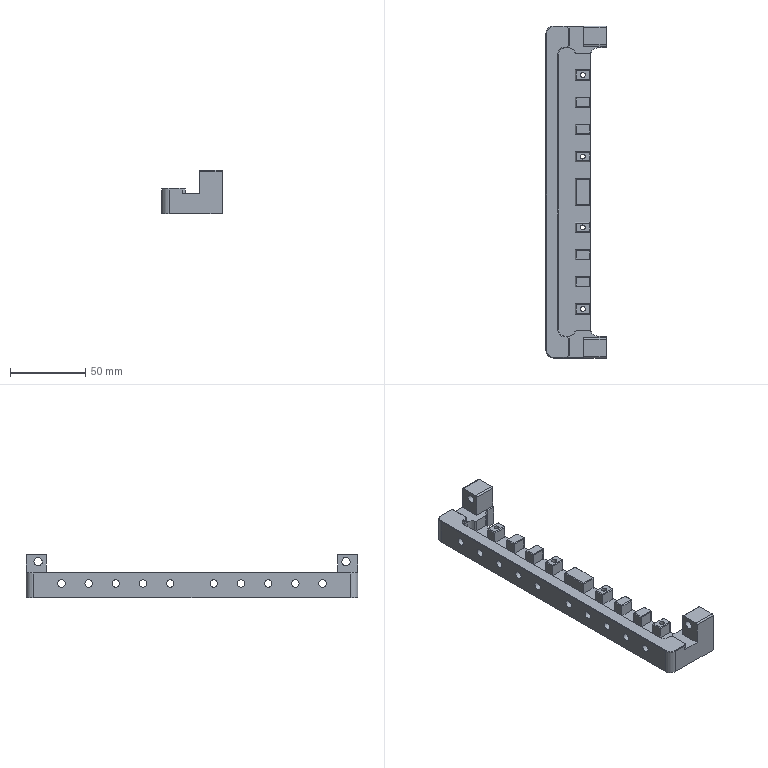CAM job | NX | 3-axis milling, drilling | part box 40 x 220 x 29 mm | stock box 45 x 225 x 35 mm
Tools:
number,name,description,diameter,corner_radius,flute_length,length,flutes
6,D6,平底铣刀-粗,6.0,0.0,25.0,75.0,2
9,D10,平底铣刀-粗,10.0,0.0,35.0,75.0,2
7,D6-J,平底铣刀-精,6.0,0.0,25.0,75.0,2
10,D10-J,平底铣刀-精,10.0,0.0,35.0,75.0,2
17,D6R0.5,圆鼻刀-粗,6.0,0.5,50.0,75.0,2
1,D80R0.8飞刀,圆鼻刀-粗,80.0,0.8,50.0,75.0,2
1,D80R0.8飞刀-J,圆鼻刀-精,80.0,0.8,50.0,75.0,2
2,D6倒角刀,倒角刀,6.0,0.0,3.0,25.0,2
21,M4X0.7,丝锥,3.3,0.0,35.0,50.0,2
13,钻头3.3,Twist Drill 3.3 mm,3.3,0.0,35.0,35.008,2
Operations:
program,operation,operation_type,tool,method,geometry_group,spindle_rpm,surface_speed,feed_per_tooth,feed_cut,feed_plunge,cut_length_mm,path_length_mm,cut_time_min,machine_time_min
B,底壁铣飞面一刀开粗_COPY,VolumeBased25DMillingOperation,D80R0.8飞刀,分层开粗-切深K-步距G,W-B,2800.0,703.696,0.5357,3000.0,100.0,3938.598,7791.555,1.313,1.698
B,底壁铣飞面一刀精光_COPY,VolumeBased25DMillingOperation,D80R0.8飞刀-J,侧刃精光-切深K-步距G,W-B,4000.0,1005.28,0.125,1000.0,100.0,328.021,364.021,0.328,0.3316
B,底壁铣分层开粗-中_COPY,VolumeBased25DMillingOperation,D10,分层开粗-切深K-步距G,W-B,8000.0,251.32,0.25,4000.0,100.0,35394.52,36209.865,8.849,8.93
B,底壁铣分层开粗-中_COPY_1,VolumeBased25DMillingOperation,D10,分层开粗-切深K-步距G,W-B,8000.0,251.32,0.25,4000.0,100.0,17945.335,18024.488,4.486,4.494
B,底壁铣分层开粗-中_COPY_2,VolumeBased25DMillingOperation,D6,分层开粗-切深K-步距G,W-B,8000.0,150.792,0.1875,3000.0,100.0,1582.336,1826.173,0.5274,0.5518
B,等高光顺清角D6参考12_COPY,ZLevelMilling,D6-J,分层精光-切深K-步距G,W-B,8000.0,150.792,0.075,1200.0,100.0,1057.613,1361.457,0.8813,0.9117
B,等高精光往复爬面_COPY,ZLevelMilling,D6R0.5,等高爬面-切深K-步距G,W-B,7000.0,131.947,0.3214,4500.0,100.0,1750.97,2143.172,0.3891,0.4283
B,钻倒角_2,Operation,D6倒角刀,METHOD,W-B,8000.0,150.796,0.0625,1000.0,0.0,20.8,276.862,0.0208,0.0464
B,平面去毛刺6X45L_COPY,SurfaceContour,D6倒角刀,爬面_倒角-切深0-步距G,W-B,6500.0,122.519,0.1154,1500.0,100.0,406.96,2498.027,0.2713,0.4804
B,平面去毛刺6X45L_COPY_1,SurfaceContour,D6倒角刀,爬面_倒角-切深0-步距G,W-B,6500.0,122.519,0.1154,1500.0,100.0,971.496,1644.992,0.6477,0.715
B,底壁铣精光底面-中_COPY,VolumeBased25DMillingOperation,D6-J,精光步距切深关,W-B,8000.0,150.792,0.0625,1000.0,100.0,74.03,133.63,0.074,0.08
B,底壁铣精光底面-中_COPY_4,VolumeBased25DMillingOperation,D6-J,精光步距切深关,W-B,7000.0,175.0,0.0536,1500.0,100.0,975.502,1028.102,0.6503,0.6556
B,底壁铣精光底面-中_COPY_3,VolumeBased25DMillingOperation,D6-J,精光步距切深关,W-B,7000.0,175.0,0.0536,1500.0,100.0,625.075,799.403,0.4167,0.4341
B,底壁铣精光底面-中_COPY_1,VolumeBased25DMillingOperation,D6-J,精光步距切深关,W-B,7000.0,175.0,0.0536,1500.0,100.0,74.03,133.63,0.0494,0.0553
B,底壁铣精光底面-中_COPY_2,VolumeBased25DMillingOperation,D6-J,精光步距切深关,W-B,8000.0,150.792,0.0625,1000.0,100.0,681.584,757.384,0.6816,0.6892
B,底壁铣精光侧面-中_COPY,VolumeBased25DMillingOperation,D6-J,侧刃精光-切深K-步距G,W-B,8000.0,150.792,0.0625,1000.0,100.0,74.707,481.632,0.0747,0.1154
B,底壁铣精光侧面-中_COPY_1,VolumeBased25DMillingOperation,D6-J,侧刃精光-切深K-步距G,W-B,8000.0,150.792,0.0625,1000.0,100.0,280.153,860.83,0.2802,0.3382
B,底壁铣精光侧面-中-选底面_COPY,VolumeBased25DMillingOperation,D6-J,侧刃精光-切深K-步距G,W-B,8000.0,150.792,0.0625,1000.0,100.0,747.836,955.024,0.7478,0.7686
A,顶面,FaceMilling,D80R0.8飞刀,侧刃精光-切深K-步距G,W-A,5000.0,1256.637,0.1,1000.0,100.0,314.0,350.0,0.314,0.3176
A,动态开粗D10_COPY,CavityMilling,D10,动态开粗-切深K-步距K,W-A,8000.0,251.32,0.25,4000.0,100.0,11970.014,12931.832,2.993,3.089
A,打点-深0.8,Operation,D6倒角刀,NONE,W-A,8000.0,150.796,0.0312,500.0,90.0,7.2,212.429,0.0144,0.0349
A,通孔-M4螺纹底孔,Operation,钻头3.3,NONE,W-A,3000.0,31.102,0.05,300.0,90.0,92.0,382.029,0.3067,0.3357
A,仅选体,SurfaceContour,D6倒角刀,METHOD,W-A,8000.0,150.796,0.1875,3000.0,100.0,549.433,585.234,0.1831,0.1867
A,钻倒角_1,Operation,D6倒角刀,METHOD,W-A,8000.0,150.796,0.0312,500.0,0.0,20.8,245.862,0.0416,0.0641
A,通孔-攻牙M4,Operation,M4X0.7,METHOD,W-A,600.0,6.22,0.0006,0.7,90.0,70.0,338.029,100.0,100.027
A,外形半精_2,VolumeBased25DMillingOperation,D10-J,METHOD,W-A,8000.0,251.327,0.0625,1000.0,100.0,1137.07,1306.079,1.137,1.154